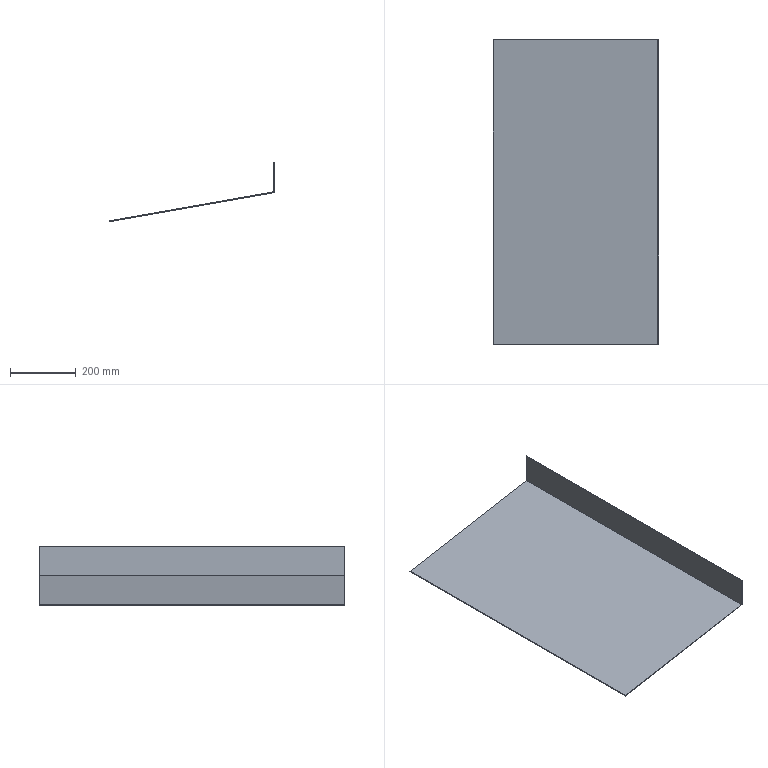Part | NX | features DATUM_CSYS 1, EXTRUDE 1, LINKED_CURVE 1 | 1 solid | 8 faces | box 503 x 926 x 181.118 mm | volume 1667441 mm3 | plane 8
STEP:
#1=CARTESIAN_POINT('',(48.,463.,-83.517));
#2=VERTEX_POINT('',#1);
#3=CARTESIAN_POINT('',(48.,463.,9.));
#4=VERTEX_POINT('',#3);
#5=CARTESIAN_POINT('',(48.,463.,-81.));
#6=DIRECTION('',(0.,0.,-1.));
#7=VECTOR('',#6,1000.);
#8=LINE('',#5,#7);
#9=EDGE_CURVE('',#2,#4,#8,.F.);
#10=ORIENTED_EDGE('',*,*,#9,.F.);
#11=CARTESIAN_POINT('',(-454.479,463.,-172.118));
#12=VERTEX_POINT('',#11);
#13=CARTESIAN_POINT('',(-454.479,463.,-172.118));
#14=DIRECTION('',(-0.9848,0.,-0.1736));
#15=VECTOR('',#14,1000.);
#16=LINE('',#13,#15);
#17=EDGE_CURVE('',#12,#2,#16,.F.);
#18=ORIENTED_EDGE('',*,*,#17,.F.);
#19=CARTESIAN_POINT('',(-455.,463.,-169.163));
#20=VERTEX_POINT('',#19);
#21=CARTESIAN_POINT('',(-455.,463.,-169.163));
#22=DIRECTION('',(0.1736,0.,-0.9848));
#23=VECTOR('',#22,1000.);
#24=LINE('',#21,#23);
#25=EDGE_CURVE('',#20,#12,#24,.T.);
#26=ORIENTED_EDGE('',*,*,#25,.F.);
#27=CARTESIAN_POINT('',(45.,463.,-81.));
#28=VERTEX_POINT('',#27);
#29=CARTESIAN_POINT('',(-455.,463.,-169.163));
#30=DIRECTION('',(0.9848,0.,0.1736));
#31=VECTOR('',#30,1000.);
#32=LINE('',#29,#31);
#33=EDGE_CURVE('',#20,#28,#32,.T.);
#34=ORIENTED_EDGE('',*,*,#33,.T.);
#35=CARTESIAN_POINT('',(45.,463.,9.));
#36=VERTEX_POINT('',#35);
#37=CARTESIAN_POINT('',(45.,463.,-81.));
#38=DIRECTION('',(0.,0.,1.));
#39=VECTOR('',#38,1000.);
#40=LINE('',#37,#39);
#41=EDGE_CURVE('',#28,#36,#40,.T.);
#42=ORIENTED_EDGE('',*,*,#41,.T.);
#43=CARTESIAN_POINT('',(45.,463.,9.));
#44=DIRECTION('',(1.,0.,0.));
#45=VECTOR('',#44,1000.);
#46=LINE('',#43,#45);
#47=EDGE_CURVE('',#36,#4,#46,.T.);
#48=ORIENTED_EDGE('',*,*,#47,.T.);
#49=EDGE_LOOP('',(#10,#18,#26,#34,#42,#48));
#50=FACE_BOUND('',#49,.T.);
#51=CARTESIAN_POINT('',(45.,463.,-81.));
#52=DIRECTION('',(0.,1.,0.));
#53=DIRECTION('',(0.,0.,1.));
#54=AXIS2_PLACEMENT_3D('',#51,#52,#53);
#55=PLANE('',#54);
#56=ADVANCED_FACE('',(#50),#55,.T.);
#57=ORIENTED_EDGE('',*,*,#47,.F.);
#58=CARTESIAN_POINT('',(45.,-463.,9.));
#59=VERTEX_POINT('',#58);
#60=CARTESIAN_POINT('',(45.,463.,9.));
#61=DIRECTION('',(0.,-1.,0.));
#62=VECTOR('',#61,1000.);
#63=LINE('',#60,#62);
#64=EDGE_CURVE('',#36,#59,#63,.T.);
#65=ORIENTED_EDGE('',*,*,#64,.T.);
#66=CARTESIAN_POINT('',(48.,-463.,9.));
#67=VERTEX_POINT('',#66);
#68=CARTESIAN_POINT('',(45.,-463.,9.));
#69=DIRECTION('',(1.,0.,0.));
#70=VECTOR('',#69,1000.);
#71=LINE('',#68,#70);
#72=EDGE_CURVE('',#59,#67,#71,.T.);
#73=ORIENTED_EDGE('',*,*,#72,.T.);
#74=CARTESIAN_POINT('',(48.,463.,9.));
#75=DIRECTION('',(0.,1.,0.));
#76=VECTOR('',#75,1000.);
#77=LINE('',#74,#76);
#78=EDGE_CURVE('',#4,#67,#77,.F.);
#79=ORIENTED_EDGE('',*,*,#78,.F.);
#80=EDGE_LOOP('',(#57,#65,#73,#79));
#81=FACE_BOUND('',#80,.T.);
#82=CARTESIAN_POINT('',(45.,463.,9.));
#83=DIRECTION('',(0.,0.,1.));
#84=DIRECTION('',(0.,-1.,0.));
#85=AXIS2_PLACEMENT_3D('',#82,#83,#84);
#86=PLANE('',#85);
#87=ADVANCED_FACE('',(#81),#86,.T.);
#88=CARTESIAN_POINT('',(-454.479,-463.,-172.118));
#89=VERTEX_POINT('',#88);
#90=CARTESIAN_POINT('',(48.,-463.,-83.517));
#91=VERTEX_POINT('',#90);
#92=CARTESIAN_POINT('',(-454.479,-463.,-172.118));
#93=DIRECTION('',(-0.9848,0.,-0.1736));
#94=VECTOR('',#93,1000.);
#95=LINE('',#92,#94);
#96=EDGE_CURVE('',#89,#91,#95,.F.);
#97=ORIENTED_EDGE('',*,*,#96,.T.);
#98=CARTESIAN_POINT('',(48.,-463.,-81.));
#99=DIRECTION('',(0.,0.,-1.));
#100=VECTOR('',#99,1000.);
#101=LINE('',#98,#100);
#102=EDGE_CURVE('',#91,#67,#101,.F.);
#103=ORIENTED_EDGE('',*,*,#102,.T.);
#104=ORIENTED_EDGE('',*,*,#72,.F.);
#105=CARTESIAN_POINT('',(45.,-463.,-81.));
#106=VERTEX_POINT('',#105);
#107=CARTESIAN_POINT('',(45.,-463.,-81.));
#108=DIRECTION('',(0.,0.,1.));
#109=VECTOR('',#108,1000.);
#110=LINE('',#107,#109);
#111=EDGE_CURVE('',#106,#59,#110,.T.);
#112=ORIENTED_EDGE('',*,*,#111,.F.);
#113=CARTESIAN_POINT('',(-455.,-463.,-169.163));
#114=VERTEX_POINT('',#113);
#115=CARTESIAN_POINT('',(-455.,-463.,-169.163));
#116=DIRECTION('',(0.9848,0.,0.1736));
#117=VECTOR('',#116,1000.);
#118=LINE('',#115,#117);
#119=EDGE_CURVE('',#114,#106,#118,.T.);
#120=ORIENTED_EDGE('',*,*,#119,.F.);
#121=CARTESIAN_POINT('',(-455.,-463.,-169.163));
#122=DIRECTION('',(0.1736,0.,-0.9848));
#123=VECTOR('',#122,1000.);
#124=LINE('',#121,#123);
#125=EDGE_CURVE('',#114,#89,#124,.T.);
#126=ORIENTED_EDGE('',*,*,#125,.T.);
#127=EDGE_LOOP('',(#97,#103,#104,#112,#120,#126));
#128=FACE_BOUND('',#127,.T.);
#129=CARTESIAN_POINT('',(-455.,-463.,-169.163));
#130=DIRECTION('',(0.,1.,0.));
#131=DIRECTION('',(0.9848,0.,0.1736));
#132=AXIS2_PLACEMENT_3D('',#129,#130,#131);
#133=PLANE('',#132);
#134=ADVANCED_FACE('',(#128),#133,.F.);
#135=CARTESIAN_POINT('',(-455.,463.,-169.163));
#136=DIRECTION('',(0.,-1.,0.));
#137=VECTOR('',#136,1000.);
#138=LINE('',#135,#137);
#139=EDGE_CURVE('',#20,#114,#138,.T.);
#140=ORIENTED_EDGE('',*,*,#139,.F.);
#141=ORIENTED_EDGE('',*,*,#25,.T.);
#142=CARTESIAN_POINT('',(-454.479,463.,-172.118));
#143=DIRECTION('',(0.,1.,0.));
#144=VECTOR('',#143,1000.);
#145=LINE('',#142,#144);
#146=EDGE_CURVE('',#12,#89,#145,.F.);
#147=ORIENTED_EDGE('',*,*,#146,.T.);
#148=ORIENTED_EDGE('',*,*,#125,.F.);
#149=EDGE_LOOP('',(#140,#141,#147,#148));
#150=FACE_BOUND('',#149,.T.);
#151=CARTESIAN_POINT('',(-455.,463.,-169.163));
#152=DIRECTION('',(0.9848,0.,0.1736));
#153=DIRECTION('',(0.,-1.,0.));
#154=AXIS2_PLACEMENT_3D('',#151,#152,#153);
#155=PLANE('',#154);
#156=ADVANCED_FACE('',(#150),#155,.F.);
#157=ORIENTED_EDGE('',*,*,#96,.F.);
#158=ORIENTED_EDGE('',*,*,#146,.F.);
#159=ORIENTED_EDGE('',*,*,#17,.T.);
#160=CARTESIAN_POINT('',(48.,463.,-83.517));
#161=DIRECTION('',(0.,-1.,0.));
#162=VECTOR('',#161,1000.);
#163=LINE('',#160,#162);
#164=EDGE_CURVE('',#2,#91,#163,.T.);
#165=ORIENTED_EDGE('',*,*,#164,.T.);
#166=EDGE_LOOP('',(#157,#158,#159,#165));
#167=FACE_BOUND('',#166,.T.);
#168=CARTESIAN_POINT('',(-454.479,463.,-172.118));
#169=DIRECTION('',(0.1736,0.,-0.9848));
#170=DIRECTION('',(-0.9848,0.,-0.1736));
#171=AXIS2_PLACEMENT_3D('',#168,#169,#170);
#172=PLANE('',#171);
#173=ADVANCED_FACE('',(#167),#172,.T.);
#174=ORIENTED_EDGE('',*,*,#102,.F.);
#175=ORIENTED_EDGE('',*,*,#164,.F.);
#176=ORIENTED_EDGE('',*,*,#9,.T.);
#177=ORIENTED_EDGE('',*,*,#78,.T.);
#178=EDGE_LOOP('',(#174,#175,#176,#177));
#179=FACE_BOUND('',#178,.T.);
#180=CARTESIAN_POINT('',(48.,463.,-81.));
#181=DIRECTION('',(1.,0.,0.));
#182=DIRECTION('',(0.,0.,-1.));
#183=AXIS2_PLACEMENT_3D('',#180,#181,#182);
#184=PLANE('',#183);
#185=ADVANCED_FACE('',(#179),#184,.T.);
#186=ORIENTED_EDGE('',*,*,#119,.T.);
#187=CARTESIAN_POINT('',(45.,463.,-81.));
#188=DIRECTION('',(0.,-1.,0.));
#189=VECTOR('',#188,1000.);
#190=LINE('',#187,#189);
#191=EDGE_CURVE('',#28,#106,#190,.T.);
#192=ORIENTED_EDGE('',*,*,#191,.F.);
#193=ORIENTED_EDGE('',*,*,#33,.F.);
#194=ORIENTED_EDGE('',*,*,#139,.T.);
#195=EDGE_LOOP('',(#186,#192,#193,#194));
#196=FACE_BOUND('',#195,.T.);
#197=CARTESIAN_POINT('',(-455.,463.,-169.163));
#198=DIRECTION('',(0.1736,0.,-0.9848));
#199=DIRECTION('',(-0.9848,0.,-0.1736));
#200=AXIS2_PLACEMENT_3D('',#197,#198,#199);
#201=PLANE('',#200);
#202=ADVANCED_FACE('',(#196),#201,.F.);
#203=ORIENTED_EDGE('',*,*,#111,.T.);
#204=ORIENTED_EDGE('',*,*,#64,.F.);
#205=ORIENTED_EDGE('',*,*,#41,.F.);
#206=ORIENTED_EDGE('',*,*,#191,.T.);
#207=EDGE_LOOP('',(#203,#204,#205,#206));
#208=FACE_BOUND('',#207,.T.);
#209=CARTESIAN_POINT('',(45.,463.,-81.));
#210=DIRECTION('',(1.,0.,0.));
#211=DIRECTION('',(0.,0.,-1.));
#212=AXIS2_PLACEMENT_3D('',#209,#210,#211);
#213=PLANE('',#212);
#214=ADVANCED_FACE('',(#208),#213,.F.);
#215=CLOSED_SHELL('',(#56,#87,#134,#156,#173,#185,#202,#214));
#216=MANIFOLD_SOLID_BREP('',#215);
#217=(LENGTH_UNIT()NAMED_UNIT(*)SI_UNIT(.MILLI.,.METRE.));
#218=UNCERTAINTY_MEASURE_WITH_UNIT(LENGTH_MEASURE(0.00001),#217,'','');
#219=(NAMED_UNIT(*)PLANE_ANGLE_UNIT()SI_UNIT($,.RADIAN.));
#220=(NAMED_UNIT(*)SI_UNIT($,.STERADIAN.)SOLID_ANGLE_UNIT());
#221=(GEOMETRIC_REPRESENTATION_CONTEXT(3)GLOBAL_UNCERTAINTY_ASSIGNED_CONTEXT((#218))GLOBAL_UNIT_ASSIGNED_CONTEXT((#217,#219,#220))REPRESENTATION_CONTEXT('',''));
#222=ADVANCED_BREP_SHAPE_REPRESENTATION('',(#216),#221);